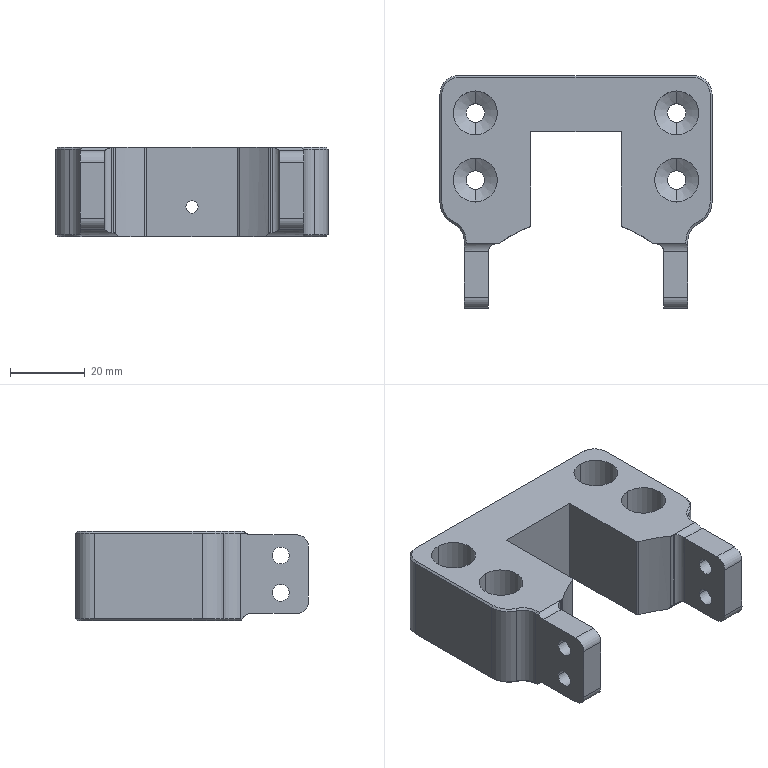NC program | NX | posted with a generic post | part box 73 x 62.4 x 24 mm
Lines 1 to 109 of 11507:
N10 G17 G21 G94 G90
(FLOOR_WALL , TOOL : D63)
N12 T01 M6
N14 G54
N16 G17 G0 G90 X-74. Y34.197 S6500 M3
N18 G43 Z30. H1
N20 Z3.
N22 G94 G1 Z0. F1250.
N24 X-71.
N26 X71.
N28 Y-9.
N30 X-71.
N32 X-74.
N34 Z3.
N36 G0 Z30.
(FLOOR_WALL_COPY_1 , TOOL : D63)
N38 G55
N40 Y34.197
N42 Z3.
N44 G1 Z0.
N46 X-71.
N48 X71.
N50 Y-9.
N52 X-71.
N54 X-74.
N56 Z3.
N58 G0 Z30.
N60 M5
(DRILLING_COPY_1 , TOOL : D6A45)
N62 T07 M6
N64 G54
N66 G17 G0 G90 X27. Y3.2 S3000 M3
N68 G43 Z30. H7
N70 G94 G81 G98 Z-1. F200. R3.
N72 Y21.2
N74 X-27.
N76 Y3.2
N78 G80
N80 G0 X-27. Y3.2 Z30.
(DRILLING_COPY_1_COPY_1 , TOOL : D6A45)
N82 G55
N84 X27.
N86 G81 Z-1. F200. R3.
N88 Y21.2
N90 X-27.
N92 Y3.2
N94 G80
N96 G0 X-27. Y3.2 Z30.
N98 M5
(DRILLING_COPY_1_COPY , TOOL : 5.0ZT)
N100 T15 M6
N102 G54
N104 G17 G0 G90 X-27. Y21.2 S2000 M3
N106 G43 Z30. H15
N108 G94 G83 G98 Z-27.002 F200. Q2. R3.
N110 Y3.2
N112 X27.
N114 Y21.2
N116 G80
N118 G0 X27. Y21.2 Z30.
(DRILLING_COPY_1_COPY_COPY_1 , TOOL : 5.0ZT)
N120 G55
N122 X-27.
N124 G83 Z-27.002 F200. Q2. R3.
N126 Y3.2
N128 X27.
N130 Y21.2
N132 G80
N134 G0 X27. Y21.2 Z30.
N136 M5
(DRILLING_COPY_1_COPY_COPY , TOOL : 11.8ZT)
N138 T12 M6
N140 G54
N142 G17 G0 G90 X-27. Y21.2 S1500 M3
N144 G43 Z30. H12
N146 G94 G83 G98 Z-18.545 F200. Q2. R3.
N148 Y3.2
N150 X27.
N152 Y21.2
N154 G80
N156 G0 X27. Y21.2 Z30.
(DRILLING_COPY_1_COPY_COPY_COPY , TOOL : 11.8ZT)
N158 G55
N160 X-27.
N162 G83 Z-18.545 F200. Q2. R3.
N164 Y3.2
N166 X27.
N168 Y21.2
N170 G80
N172 G0 X27. Y21.2 Z30.
N174 M5